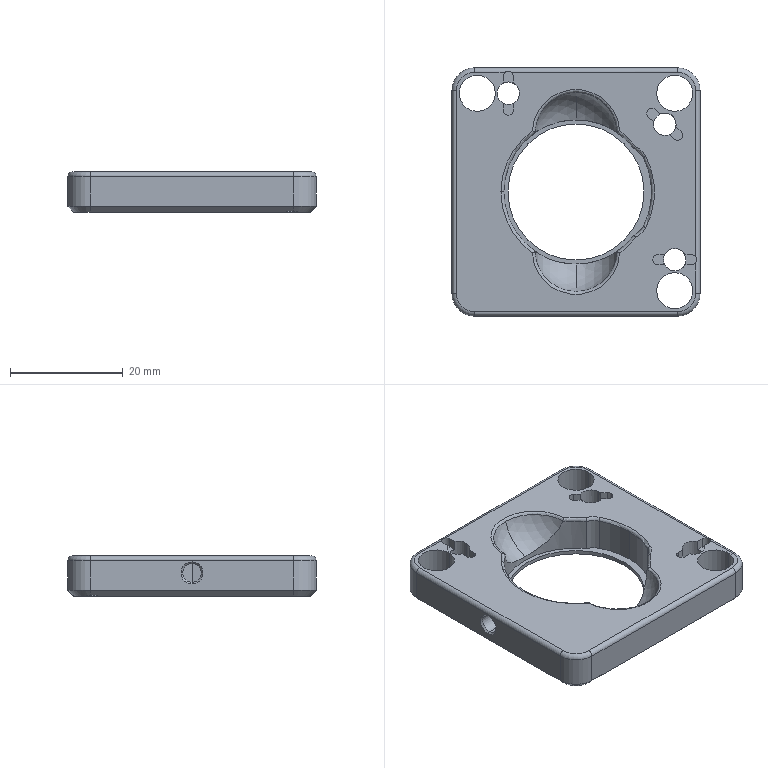Part | STEP file | 1 solid | 107 faces | box 44 x 44 x 7.1 mm | volume 8399 mm3 | cylinder 43 | plane 41 | torus 13 | cone 6 | sphere 4 | commonest cylinder face diameters 1.8 x8 4 x6 6.4 x6 7.3 x6 1.6 x4 8 x4